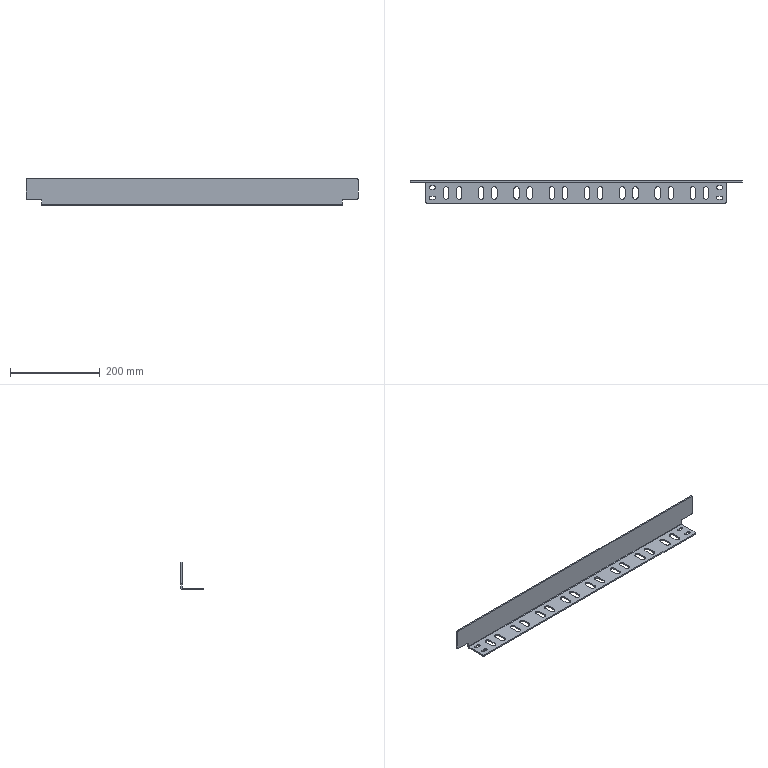Part | SolidWorks | features BaseBody 1 | 1 solid | 110 faces | box 739 x 50 x 62 mm | volume 210888 mm3 | plane 56 | cylinder 54 | commonest cylinder face diameters 12 x32 7 x12 6 x8 2 x1 8 x1